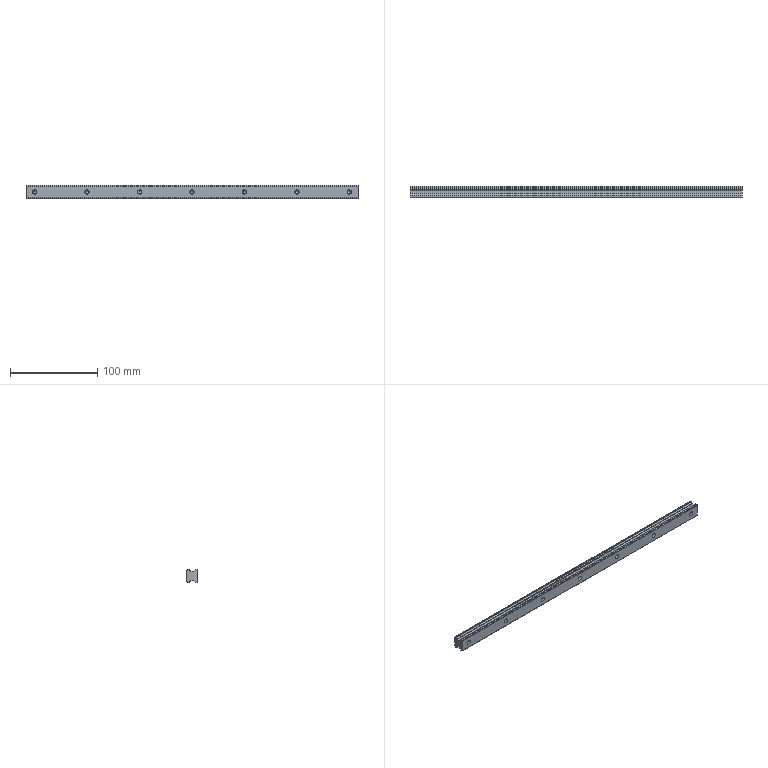Part | STEP file | J454-EBZ05-98-04-Part-1 | 1 solid | 94 faces | box 380 x 13 x 15 mm | volume 62425 mm3 | cylinder 51 | plane 29 | cone 14 | commonest cylinder face diameters 4.134 x14 5 x14 0.6 x6 2.861 x4 0.398 x3 0.545 x2